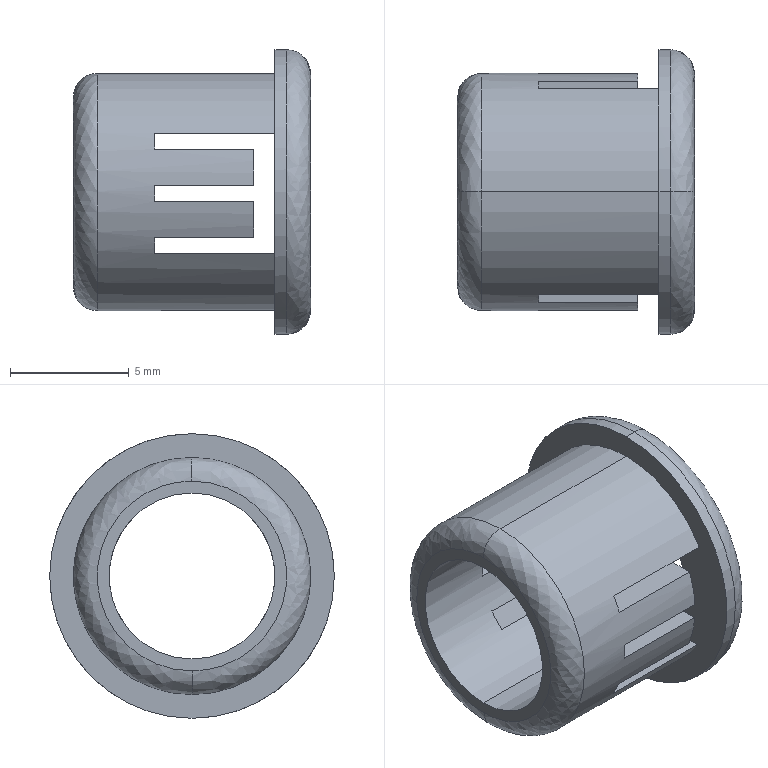Part | STEP file | 1 solid | 35 faces | box 10 x 12 x 12 mm | volume 394.73 mm3 | plane 25 | cylinder 6 | spline 4 | commonest cylinder face diameters 7 x2 10 x2 12 x2